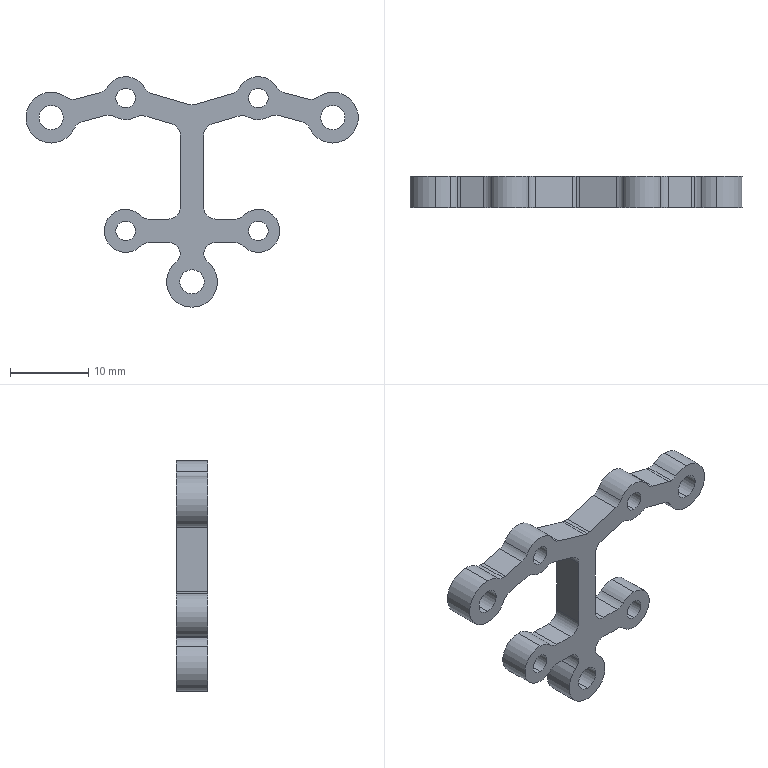Part | SolidWorks | features Extrusion 1, Fillet 1, HoleWzd 1 | 1 solid | 78 faces | box 42.5 x 4 x 29.485 mm | volume 1175 mm3 | cylinder 62 | plane 16 | commonest cylinder face diameters 3 x28 5.5 x12 2.5 x8 6.5 x8 3.1 x6